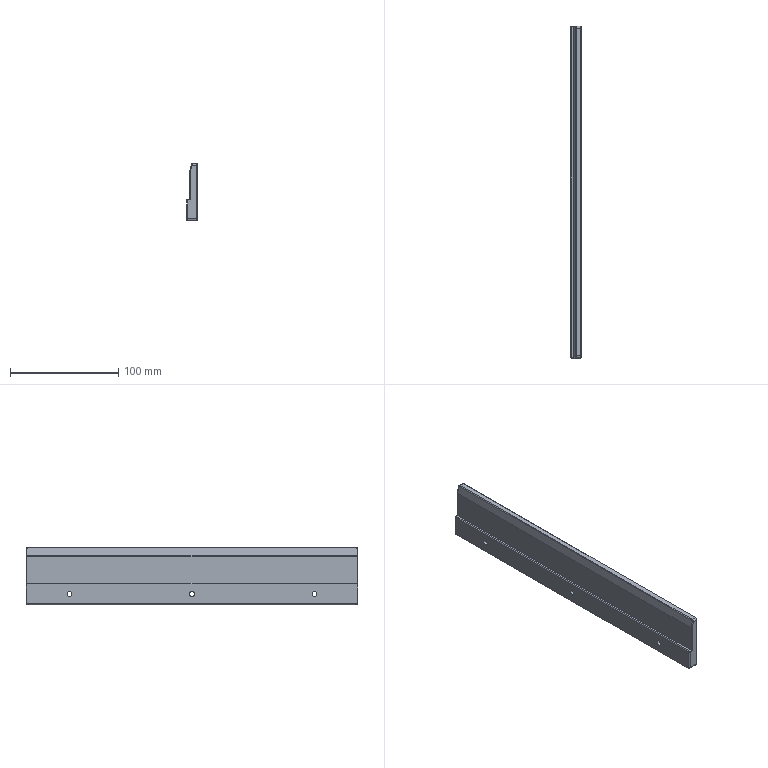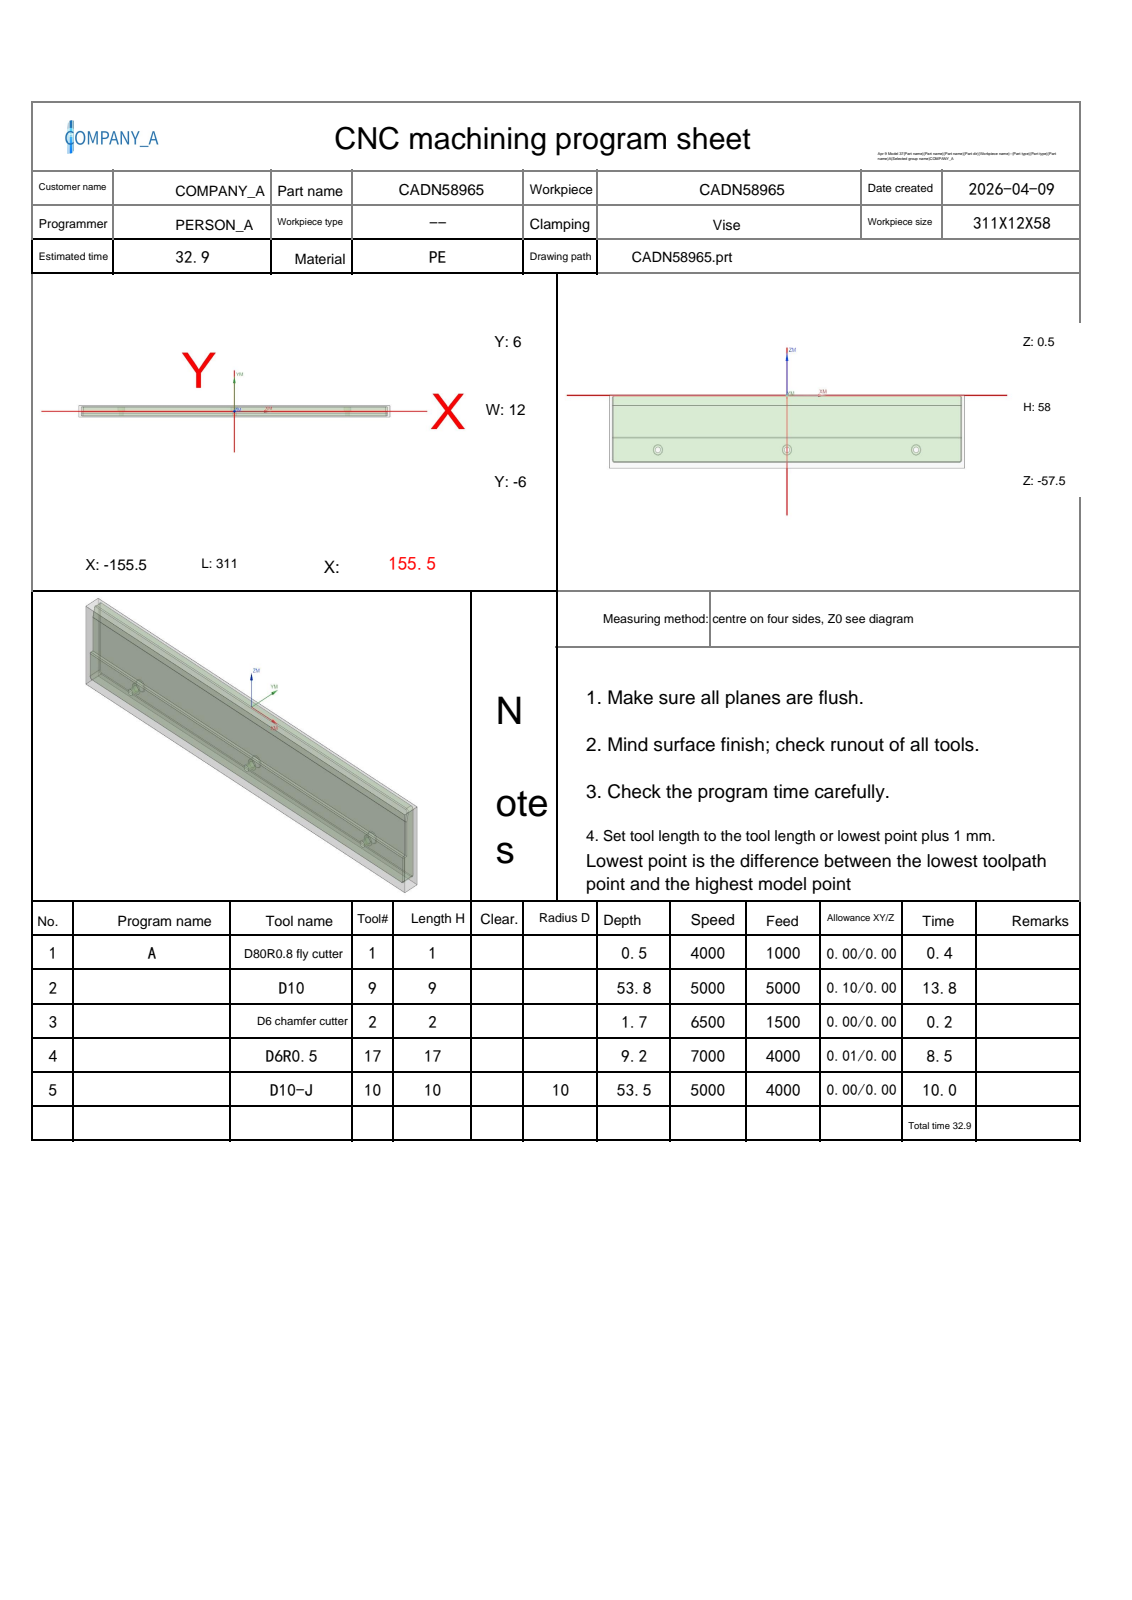NC program | NX | posted by the shop | part box 10 x 306 x 53 mm
Lines 3099 to 3792 of 3792:
N5 T10 M06
(D10-J  D=10. R=0. H=10 ce=0.00 di=0.00)
G00 G90 G54 X153.763 Y-8.844 M03 S5000
G43 H10 Z5.5
M08
Z-7.833
G01 Z-8.833 F1000.
G41 D10
X153.742 Y-8.645
G03 X152.25 Y-7.3 I-1.492 J-.155
G01 X-152.25
G02 X-158. Y-1.55 I0.0 J5.75
G01 Y4.5
G02 X-156.536 Y8.036 I5. J0.0
G01 X-156.036 Y8.536
G02 X-152.5 Y10. I3.536 J-3.536
G01 X152.5
G02 X156.036 Y8.536 I0.0 J-5.
G01 X156.536 Y8.036
G02 X158. Y4.5 I-3.536 J-3.536
G01 Y-1.55
G02 X152.25 Y-7.3 I-5.75 J0.0
G03 X150.75 Y-8.8 I0.0 J-1.5
G01 G40 Y-9.
Z-7.833
G00 X153.763 Y-8.844
Z-16.667
G01 Z-17.667
G41 D10
X153.742 Y-8.645
G03 X152.25 Y-7.3 I-1.492 J-.155
G01 X-152.25
G02 X-158. Y-1.55 I0.0 J5.75
G01 Y4.5
G02 X-156.536 Y8.036 I5. J0.0
G01 X-156.036 Y8.536
G02 X-152.5 Y10. I3.536 J-3.536
G01 X152.5
G02 X156.036 Y8.536 I0.0 J-5.
G01 X156.536 Y8.036
G02 X158. Y4.5 I-3.536 J-3.536
G01 Y-1.55
G02 X152.25 Y-7.3 I-5.75 J0.0
G03 X150.75 Y-8.8 I0.0 J-1.5
G01 G40 Y-9.
Z-16.667
G00 X153.763 Y-8.844
Z-25.5
G01 Z-26.5
G41 D10
X153.742 Y-8.645
G03 X152.25 Y-7.3 I-1.492 J-.155
G01 X-152.25
G02 X-158. Y-1.55 I0.0 J5.75
G01 Y4.5
G02 X-156.536 Y8.036 I5. J0.0
G01 X-156.036 Y8.536
G02 X-152.5 Y10. I3.536 J-3.536
G01 X152.5
G02 X156.036 Y8.536 I0.0 J-5.
G01 X156.536 Y8.036
G02 X158. Y4.5 I-3.536 J-3.536
G01 Y-1.55
G02 X152.25 Y-7.3 I-5.75 J0.0
G03 X150.75 Y-8.8 I0.0 J-1.5
G01 G40 Y-9.
Z-25.5
G00 X153.763 Y-11.544
Z-34.333
G01 Z-35.333
G41 D10
X153.742 Y-11.345
G03 X152.25 Y-10. I-1.492 J-.155
G01 X-152.25
G02 X-158. Y-4.25 I0.0 J5.75
G01 Y4.5
G02 X-156.536 Y8.036 I5. J0.0
G01 X-156.036 Y8.536
G02 X-152.5 Y10. I3.536 J-3.536
G01 X152.5
G02 X156.036 Y8.536 I0.0 J-5.
G01 X156.536 Y8.036
G02 X158. Y4.5 I-3.536 J-3.536
G01 Y-4.25
G02 X152.25 Y-10. I-5.75 J0.0
G03 X150.75 Y-11.5 I0.0 J-1.5
G01 G40 Y-11.7
Z-34.333
G00 Z5.5
X159.338 Y-3.842
Z-32.
G01 Z-33.
G41 D10
X159.155 Y-3.761
G03 X158.552 Y-3.635 I-.603 J-1.374
X157.248 Y-4.393 I0.0 J-1.5
G02 X152.25 Y-7.3 I-4.998 J2.843
G01 X-152.25
G02 X-157.248 Y-4.393 I0.0 J5.75
G03 X-158.552 Y-3.635 I-1.304 J-.742
X-159.155 Y-3.761 I0.0 J-1.5
G01 G40 X-159.338 Y-3.842
Z-32.
G00 Z5.5
X-154.013 Y11.526
Z-43.167
G01 Z-44.167
G41 D10
X-153.99 Y11.327
G03 X-152.5 Y10. I1.49 J.173
G01 X152.5
G02 X156.036 Y8.536 I0.0 J-5.
G01 X156.536 Y8.036
G02 X158. Y4.5 I-3.536 J-3.536
G01 Y-4.25
G02 X152.25 Y-10. I-5.75 J0.0
G01 X-152.25
G02 X-158. Y-4.25 I0.0 J5.75
G01 Y4.5
G02 X-156.536 Y8.036 I5. J0.0
G01 X-156.036 Y8.536
G02 X-152.5 Y10. I3.536 J-3.536
G03 X-151. Y11.5 I0.0 J1.5
G01 G40 Y11.7
Z-43.167
G00 X-154.013 Y11.526
Z-52.
G01 Z-53.
G41 D10
X-153.99 Y11.327
G03 X-152.5 Y10. I1.49 J.173
G01 X152.5
G02 X156.036 Y8.536 I0.0 J-5.
G01 X156.536 Y8.036
G02 X158. Y4.5 I-3.536 J-3.536
G01 Y-4.25
G02 X152.25 Y-10. I-5.75 J0.0
G01 X-152.25
G02 X-158. Y-4.25 I0.0 J5.75
G01 Y4.5
G02 X-156.536 Y8.036 I5. J0.0
G01 X-156.036 Y8.536
G02 X-152.5 Y10. I3.536 J-3.536
G03 X-151. Y11.5 I0.0 J1.5
G01 G40 Y11.7
Z-52.
G00 Z5.5
G00 G90 X163.01 Y-1.499 M03 S5000
Z10.5
Z-32.508
G01 Z-33.008 F4000.
G03 X161.871 Y-1.368 I-1.139 J-4.868
X157.375 Y-4.179 I0.0 J-5.
G01 X157.369 Y-4.191
Y-4.25
G02 X152.25 Y-9.369 I-5.119 J0.0
G01 X-152.25
G02 X-157.369 Y-4.25 I0.0 J5.119
G01 Y-4.191
X-157.375 Y-4.179
X-157.397 Y-4.135 Z-33.012
X-157.393 Y-4.145
X-157.394 Y-4.25
G03 X-152.25 Y-9.394 I5.144 J0.0
G01 X152.25
G03 X157.394 Y-4.25 I0.0 J5.144
G01 X157.393 Y-4.145
X157.397 Y-4.135
X157.421 Y-4.088 Z-33.016
X157.414 Y-4.107
Y-4.25
G02 X152.25 Y-9.414 I-5.164 J0.0
G01 X-152.25
G02 X-157.414 Y-4.25 I0.0 J5.164
G01 Y-4.107
X-157.421 Y-4.088
X-157.432 Y-4.065 Z-33.02
X-157.423 Y-4.22
X-157.432 Y-4.25
G03 X-152.25 Y-9.432 I5.182 J0.0
G01 X152.25
G03 X157.432 Y-4.25 I0.0 J5.182
G01 Y-4.065
X157.454 Y-4.02 Z-33.024
X157.449 Y-4.032
Y-4.25
G02 X152.25 Y-9.449 I-5.199 J0.0
G01 X-152.25
G02 X-157.449 Y-4.25 I0.0 J5.199
G01 X-157.441 Y-4.23
X-157.449 Y-4.032
X-157.454 Y-4.02
X-157.464 Y-3.997 Z-33.028
X-157.46 Y-4.24
X-157.464 Y-4.25
G03 X-152.25 Y-9.464 I5.214 J0.0
G01 X152.25
G03 X157.464 Y-4.25 I0.0 J5.214
G01 Y-3.997
X157.48 Y-3.963 Z-33.033
Y-4.25
G02 X152.25 Y-9.48 I-5.23 J0.0
G01 X-152.25
G02 X-157.48 Y-4.25 I0.0 J5.23
G01 Y-3.963
X-157.496 Y-3.929 Z-33.038
X-157.487 Y-4.195
X-157.495 Y-4.25
G03 X-152.25 Y-9.495 I5.245 J0.0
G01 X152.25
G03 X157.495 Y-4.25 I0.0 J5.245
G01 X157.496 Y-3.929
X157.511 Y-3.894 Z-33.043
X157.51 Y-4.25
G02 X152.25 Y-9.51 I-5.26 J0.0
G01 X-152.25
G02 X-157.51 Y-4.25 I0.0 J5.26
G01 X-157.505 Y-4.206
X-157.51 Y-3.907
X-157.511 Y-3.894
X-157.525 Y-3.863 Z-33.048
Y-4.25
G03 X-152.25 Y-9.525 I5.275 J0.0
G01 X152.25
G03 X157.525 Y-4.25 I0.0 J5.275
G01 Y-3.863
X157.543 Y-3.822 Z-33.054
X157.539 Y-3.835
Y-4.25
G02 X152.25 Y-9.539 I-5.289 J0.0
G01 X-152.25
G02 X-157.539 Y-4.25 I0.0 J5.289
G01 Y-3.835
X-157.543 Y-3.822
X-157.554 Y-3.797 Z-33.06
Y-4.25
G03 X-152.25 Y-9.554 I5.304 J0.0
G01 X152.25
G03 X157.554 Y-4.25 I0.0 J5.304
G01 Y-3.797
X157.57 Y-3.758 Z-33.066
X157.566 Y-3.817
X157.568 Y-4.25
G02 X152.25 Y-9.568 I-5.318 J0.0
G01 X-152.25
G02 X-157.568 Y-4.25 I0.0 J5.318
G01 X-157.57 Y-3.758
X-157.586 Y-3.72 Z-33.073
X-157.582 Y-3.733
Y-4.25
G03 X-152.25 Y-9.582 I5.332 J0.0
G01 X152.25
G03 X157.582 Y-4.25 I0.0 J5.332
G01 Y-3.733
X157.586 Y-3.72
X157.596 Y-3.694 Z-33.079
Y-4.25
G02 X152.25 Y-9.596 I-5.346 J0.0
G01 X-152.25
G02 X-157.596 Y-4.25 I0.0 J5.346
G01 Y-3.694
X-157.611 Y-3.656 Z-33.087
X-157.61 Y-3.67
Y-4.25
G03 X-152.25 Y-9.61 I5.36 J0.0
G01 X152.25
G03 X157.61 Y-4.25 I0.0 J5.36
G01 Y-3.67
X157.611 Y-3.656
X157.623 Y-3.626 Z-33.094
Y-4.25
G02 X152.25 Y-9.623 I-5.373 J0.0
G01 X-152.25
G02 X-157.623 Y-4.25 I0.0 J5.373
G01 Y-3.625
X-157.638 Y-3.585 Z-33.101
X-157.636 Y-3.6
X-157.637 Y-4.25
G03 X-152.25 Y-9.637 I5.387 J0.0
G01 X152.25
G03 X157.637 Y-4.25 I0.0 J5.387
G01 X157.636 Y-3.602
X157.638 Y-3.587
X157.652 Y-3.549 Z-33.109
X157.649 Y-3.562
X157.65 Y-4.25
G02 X152.25 Y-9.65 I-5.4 J0.0
G01 X-152.25
G02 X-157.65 Y-4.25 I0.0 J5.4
G01 Y-3.56
X-157.653 Y-3.546
X-157.663 Y-3.52 Z-33.117
X-157.659 Y-3.653
X-157.663 Y-4.25
G03 X-152.25 Y-9.663 I5.413 J0.0
G01 X152.25
G03 X157.663 Y-4.25 I0.0 J5.413
G01 Y-3.523
X157.666 Y-3.509
X157.676 Y-3.483 Z-33.126
X157.675 Y-4.25
G02 X152.25 Y-9.675 I-5.425 J0.0
G01 X-152.25
G02 X-157.675 Y-4.25 I0.0 J5.425
G01 X-157.677 Y-3.481
X-157.691 Y-3.441 Z-33.134
X-157.688 Y-3.455
Y-4.25
G03 X-152.25 Y-9.688 I5.438 J0.0
G01 X152.25
G03 X157.688 Y-4.25 I0.0 J5.438
G01 X157.69 Y-3.444
X157.704 Y-3.403 Z-33.143
X157.701 Y-4.25
G02 X152.25 Y-9.701 I-5.451 J0.0
G01 X-152.25
G02 X-157.701 Y-4.25 I0.0 J5.451
G01 Y-3.415
X-157.704 Y-3.403
X-157.713 Y-3.375 Z-33.152
Y-4.25
G03 X-152.25 Y-9.713 I5.463 J0.0
G01 X152.25
G03 X157.713 Y-4.25 I0.0 J5.463
G01 Y-3.378
X157.717 Y-3.365
X157.725 Y-3.338 Z-33.161
X157.722 Y-3.423
X157.725 Y-4.25
G02 X152.25 Y-9.725 I-5.475 J0.0
G01 X-152.25
G02 X-157.725 Y-4.25 I0.0 J5.475
G01 X-157.726 Y-3.336
X-157.739 Y-3.296 Z-33.171
X-157.736 Y-3.31
X-157.734 Y-4.065
X-157.737 Y-4.25
G03 X-152.25 Y-9.737 I5.487 J0.0
G01 X152.25
G03 X157.737 Y-4.25 I0.0 J5.487
G01 X157.733 Y-3.427
X157.738 Y-3.298
X157.751 Y-3.258 Z-33.181
X157.744 Y-3.431
X157.748 Y-4.25
G02 X152.25 Y-9.748 I-5.498 J0.0
G01 X-152.25
G02 X-157.748 Y-4.25 I0.0 J5.498
G01 X-157.747 Y-3.269
X-157.76 Y-3.229 Z-33.191
X-157.758 Y-4.065
X-157.76 Y-4.25
G03 X-152.25 Y-9.76 I5.51 J0.0
G01 X152.25
G03 X157.76 Y-4.25 I0.0 J5.51
G01 X157.758 Y-4.065
X157.759 Y-3.231
X157.771 Y-3.191 Z-33.201
X157.767 Y-4.065
X157.771 Y-4.25
G02 X152.25 Y-9.771 I-5.521 J0.0
G01 X-152.25
G02 X-157.771 Y-4.25 I0.0 J5.521
G01 X-157.767 Y-4.065
X-157.772 Y-3.189
X-157.784 Y-3.149 Z-33.211
X-157.777 Y-4.065
X-157.782 Y-4.25
G03 X-152.25 Y-9.782 I5.532 J0.0
G01 X152.25
G03 X157.782 Y-4.25 I0.0 J5.532
G01 X157.777 Y-4.065
X157.783 Y-3.15
X157.793 Y-3.139 Z-33.222
Y-4.25
G02 X152.25 Y-9.793 I-5.543 J0.0
G01 X-152.25
G02 X-157.793 Y-4.25 I0.0 J5.543
G01 X-157.787 Y-3.136
X-157.803 Y-3.146 Z-33.233
Y-4.25
G03 X-152.25 Y-9.803 I5.553 J0.0
G01 X152.25
G03 X157.803 Y-4.25 I0.0 J5.553
G01 Y-3.143
X157.813 Y-3.146 Z-33.244
Y-4.25
G02 X152.25 Y-9.813 I-5.563 J0.0
G01 X-152.25
G02 X-157.813 Y-4.25 I0.0 J5.563
G01 Y-3.148
X-157.824 Y-3.137 Z-33.255
Y-4.25
G03 X-152.25 Y-9.824 I5.574 J0.0
G01 X152.25
G03 X157.824 Y-4.25 I0.0 J5.574
G01 Y-3.149
X157.833 Y-3.136 Z-33.267
Y-4.25
G02 X152.25 Y-9.833 I-5.583 J0.0
G01 X-152.25
G02 X-157.833 Y-4.25 I0.0 J5.583
G01 Y-3.14
X-157.843 Y-3.143 Z-33.278
Y-4.25
G03 X-152.25 Y-9.843 I5.593 J0.0
G01 X152.25
G03 X157.843 Y-4.25 I0.0 J5.593
G01 Y-3.139
X157.852 Y-3.141 Z-33.29
Y-4.25
G02 X152.25 Y-9.852 I-5.602 J0.0
G01 X-152.25
G02 X-157.852 Y-4.25 I0.0 J5.602
G01 Y-3.145
X-157.862 Y-3.148 Z-33.302
Y-4.25
G03 X-152.25 Y-9.862 I5.612 J0.0
G01 X152.25
G03 X157.862 Y-4.25 I0.0 J5.612
G01 Y-3.144
X157.87 Y-3.146 Z-33.314
Y-4.25
G02 X152.25 Y-9.87 I-5.62 J0.0
G01 X-152.25
G02 X-157.87 Y-4.25 I0.0 J5.62
G01 Y-3.15
X-157.879 Y-3.138 Z-33.327
Y-4.25
G03 X-152.25 Y-9.879 I5.629 J0.0
G01 X152.25
G03 X157.879 Y-4.25 I0.0 J5.629
G01 Y-3.148
X157.887 Y-3.14 Z-33.339
Y-4.25
G02 X152.25 Y-9.887 I-5.637 J0.0
G01 X-152.25
G02 X-157.887 Y-4.25 I0.0 J5.637
G01 Y-3.14
X-157.896 Z-33.352
Y-4.25
G03 X-152.25 Y-9.896 I5.646 J0.0
G01 X152.25
G03 X157.896 Y-4.25 I0.0 J5.646
G01 Y-3.14
X157.903 Z-33.365
Y-4.25
G02 X152.25 Y-9.903 I-5.653 J0.0
G01 X-152.25
G02 X-157.903 Y-4.25 I0.0 J5.653
G01 Y-3.14
X-157.911 Z-33.378
X-157.91 Y-3.151
Y-4.065
X-157.911 Y-4.25
G03 X-152.25 Y-9.911 I5.661 J0.0
G01 X152.25
G03 X157.911 Y-4.25 I0.0 J5.661
G01 X157.905 Y-3.151
X157.911 Y-3.14
X157.918 Z-33.391
G03 X157.91 Y-3.654 I16.353 J-.514
X157.916 Y-4.097 I16.361 J0.0
G01 X157.918 Y-4.25
G02 X152.25 Y-9.918 I-5.668 J0.0
G01 X-152.25
G02 X-157.918 Y-4.25 I0.0 J5.668
G01 X-157.916 Y-4.097
G03 X-157.91 Y-3.654 I-16.366 J.443
X-157.918 Y-3.14 I-16.372 J0.0
G01 X-157.925 Z-33.404
G02 X-157.917 Y-3.649 I-14.493 J-.509
X-157.923 Y-4.081 I-14.502 J0.0
G01 X-157.925 Y-4.25
G03 X-152.25 Y-9.925 I5.675 J0.0
G01 X152.25
G03 X157.925 Y-4.25 I0.0 J5.675
G01 X157.923 Y-4.081
G02 X157.917 Y-3.649 I14.495 J.432
X157.925 Y-3.14 I14.502 J0.0
G01 X157.932 Z-33.418
G03 X157.923 Y-3.647 I13.656 J-.507
X157.93 Y-4.073 I13.666 J0.0
G01 X157.932 Y-4.25
G02 X152.25 Y-9.932 I-5.682 J0.0
G01 X-152.25
G02 X-157.932 Y-4.25 I0.0 J5.682
G01 X-157.93 Y-4.073
G03 X-157.923 Y-3.647 I-13.659 J.426
X-157.932 Y-3.14 I-13.666 J0.0
G01 X-157.939 Z-33.431
G02 X-157.929 Y-3.646 I-13.575 J-.507
X-157.936 Y-4.072 I-13.585 J0.0
G01 X-157.939 Y-4.25
G03 X-152.25 Y-9.939 I5.689 J0.0
G01 X152.25
G03 X157.939 Y-4.25 I0.0 J5.689
G01 X157.936 Y-4.072
G02 X157.929 Y-3.646 I13.582 J.426
X157.939 Y-3.14 I13.589 J0.0
G01 X157.945 Z-33.445
G03 X157.936 Y-3.648 I14.341 J-.509
X157.943 Y-4.079 I14.35 J0.0
G01 X157.945 Y-4.25
G02 X152.25 Y-9.945 I-5.695 J0.0
G01 X-152.25
G02 X-157.945 Y-4.25 I0.0 J5.695
G01 X-157.942 Y-4.078
G03 X-157.936 Y-3.648 I-14.222 J.43
X-157.945 Y-3.14 I-14.228 J0.0
G01 X-157.951 Z-33.459
X-157.949 Y-3.151
X-157.948 Y-4.065
X-157.951 Y-4.25
G03 X-152.25 Y-9.951 I5.701 J0.0
G01 X152.25
G03 X157.951 Y-4.25 I0.0 J5.701
G01 X157.948 Y-4.065
X157.945 Y-3.151
X157.951 Y-3.14
X157.957 Z-33.473
X157.951 Y-3.151
X157.954 Y-4.065
X157.957 Y-4.25
G02 X152.25 Y-9.957 I-5.707 J0.0
G01 X-152.25
G02 X-157.957 Y-4.25 I0.0 J5.707
G01 X-157.954 Y-3.151
X-157.957 Y-3.14
X-157.962 Z-33.487
Y-4.25
G03 X-152.25 Y-9.962 I5.712 J0.0
G01 X152.25
G03 X157.962 Y-4.25 I0.0 J5.712
G01 Y-3.14
X157.967 Z-33.501
Y-4.25
G02 X152.25 Y-9.967 I-5.717 J0.0
G01 X-152.25
G02 X-157.967 Y-4.25 I0.0 J5.717
G01 Y-3.14
X-157.972 Z-33.515
Y-4.25
G03 X-152.25 Y-9.972 I5.722 J0.0
G01 X152.25
G03 X157.972 Y-4.25 I0.0 J5.722
G01 Y-3.14
X157.977 Y-3.142 Z-33.529
Y-4.25
G02 X152.25 Y-9.977 I-5.727 J0.0
G01 X-152.25
G02 X-157.977 Y-4.25 I0.0 J5.727
G01 Y-3.142
X-157.981 Z-33.544
Y-4.25
G03 X-152.25 Y-9.981 I5.731 J0.0
G01 X152.25
G03 X157.981 Y-4.25 I0.0 J5.731
G01 Y-3.142
X157.985 Z-33.558
Y-4.25
G02 X152.25 Y-9.985 I-5.735 J0.0
G01 X-152.25
G02 X-157.985 Y-4.25 I0.0 J5.735
G01 Y-3.142
X-157.989 Z-33.573
Y-4.25
G03 X-152.25 Y-9.989 I5.739 J0.0
G01 X152.25
G03 X157.989 Y-4.25 I0.0 J5.739
G01 Y-3.142
X157.992 Z-33.587
Y-4.25
G02 X152.25 Y-9.992 I-5.742 J0.0
G01 X-152.25
G02 X-157.992 Y-4.25 I0.0 J5.742
G01 Y-3.142
X-157.995 Z-33.602
Y-4.25
G03 X-152.25 Y-9.995 I5.745 J0.0
G01 X152.25
G03 X157.995 Y-4.25 I0.0 J5.745
G01 Y-3.142
X157.998 Z-33.617
Y-4.25
G02 X152.25 Y-9.998 I-5.748 J0.0
G01 X-152.25
G02 X-157.998 Y-4.25 I0.0 J5.748
G01 Y-3.142
X-158.001 Z-33.632
Y-4.25
G03 X-152.25 Y-10.001 I5.751 J0.0
G01 X152.25
G03 X158.001 Y-4.25 I0.0 J5.751
G01 Y-3.142
X158.003 Z-33.646
Y-4.25
G02 X152.25 Y-10.003 I-5.753 J0.0
G01 X-152.25
G02 X-158.003 Y-4.25 I0.0 J5.753
G01 Y-3.142
X-158.005 Z-33.661
Y-4.25
G03 X-152.25 Y-10.005 I5.755 J0.0
G01 X152.25
G03 X158.005 Y-4.25 I0.0 J5.755
G01 Y-3.142
X158.006 Z-33.676
Y-4.25
G02 X152.25 Y-10.006 I-5.756 J0.0
G01 X-152.25
G02 X-158.006 Y-4.25 I0.0 J5.756
G01 Y-3.142
X-158.008 Z-33.691
Y-4.25
G03 X-152.25 Y-10.008 I5.758 J0.0
G01 X152.25
G03 X158.008 Y-4.25 I0.0 J5.758
G01 Y-3.142
X158.009 Z-33.706
Y-4.25
G02 X152.25 Y-10.009 I-5.759 J0.0
G01 X-152.25
G02 X-158.009 Y-4.25 I0.0 J5.759
G01 Y-3.142
Z-33.721
Y-4.285
G03 X-157.883 Y-5.448 I5.759 J.035
G01 X-157.857 Y-5.56
X-157.721 Y-6.049
G03 X-155.721 Y-8.846 I5.471 J1.799
G01 X-155.485 Y-9.015
X-155.437 Y-9.047
G03 X-154.604 Y-9.507 I3.187 J4.797
G01 X-154.536 Y-9.536
G03 X-153.683 Y-9.828 I2.286 J5.286
G01 X-153.263 Y-9.92
G03 X-152.25 Y-10.009 I1.013 J5.67
G01 X152.25
G03 X153.263 Y-9.92 I0.0 J5.759
G01 X153.61 Y-9.846
G03 X154.536 Y-9.536 I-1.36 J5.596
G01 X154.604 Y-9.507
G03 X155.485 Y-9.015 I-2.354 J5.257
G01 X155.721 Y-8.846
G03 X158.009 Y-4.285 I-3.471 J4.596
G01 Y-3.142
X158.01 Z-33.736
X158.009 Y-4.353
G02 X157.097 Y-7.362 I-5.759 J.103
G01 X157.079 Y-7.389
G02 X156.456 Y-8.185 I-4.829 J3.139
G01 X156.219 Y-8.424
G02 X153.247 Y-9.923 I-3.969 J4.174
X152.356 Y-10.008 I-.991 J5.674
G01 X152.25 Y-10.01
X-152.27
X-152.37 Y-10.009
G02 X-154.604 Y-9.507 I.12 J5.759
X-155.389 Y-9.079 I2.356 J5.256
G01 X-155.722 Y-8.846
G02 X-156.233 Y-8.41 I3.473 J4.595
G01 X-156.456 Y-8.185
G02 X-157.079 Y-7.389 I4.206 J3.935
G01 X-157.097 Y-7.362
G02 X-158.009 Y-4.353 I4.847 J3.112
G01 X-158.01 Y-3.142
Y-3.148 Z-33.75
X-158.009 Y-4.353
G03 X-157.097 Y-7.362 I5.759 J.103
G01 X-157.079 Y-7.39
G03 X-156.456 Y-8.185 I4.829 J3.14
G01 X-156.219 Y-8.424
G03 X-155.722 Y-8.846 I3.969 J4.174
G01 X-155.437 Y-9.047
X-155.365 Y-9.095
G03 X-152.37 Y-10.009 I3.115 J4.845
G01 X-152.356 Y-10.008
X-152.27 Y-10.01
X152.25
X152.37 Y-10.009
G03 X156.219 Y-8.424 I-.12 J5.759
G01 X156.456 Y-8.185
G03 X157.079 Y-7.39 I-4.206 J3.935
G01 X157.097 Y-7.362
G03 X158.009 Y-4.353 I-4.847 J3.112
G01 X158.01 Y-3.148
G00 Z10.5
M05
M09
G91 G28 Z0.0
G91 G28 Y0.0
M30
%